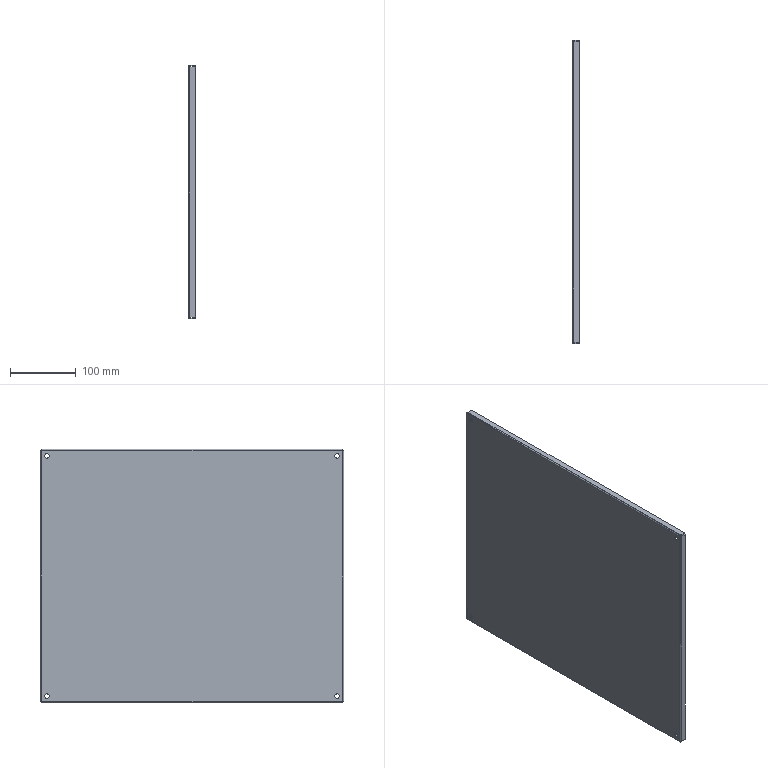Part | SolidWorks | features BaseBody 1 | 1 solid | 38 faces | box 10 x 462 x 386 mm | volume 287636 mm3 | plane 22 | cylinder 16 | commonest cylinder face diameters 7 x8 0.4 x4 3.4 x4
STEP:
#1=CARTESIAN_POINT('',(1256.5,54.,45.5));
#2=VERTEX_POINT('',#1);
#3=CARTESIAN_POINT('',(1256.5,54.,38.5));
#4=VERTEX_POINT('',#3);
#5=CARTESIAN_POINT('',(1256.5,54.,42.));
#6=DIRECTION('',(1.,0.,0.));
#7=DIRECTION('',(0.,0.,-1.));
#8=AXIS2_PLACEMENT_3D('',#5,#6,#7);
#9=CIRCLE('',#8,3.5);
#10=EDGE_CURVE('',#2,#4,#9,.T.);
#11=ORIENTED_EDGE('',*,*,#10,.T.);
#12=CARTESIAN_POINT('',(1255.,54.,38.5));
#13=VERTEX_POINT('',#12);
#14=CARTESIAN_POINT('',(1255.,54.,38.5));
#15=DIRECTION('',(-1.,0.,0.));
#16=VECTOR('',#15,1000.);
#17=LINE('',#14,#16);
#18=EDGE_CURVE('',#4,#13,#17,.T.);
#19=ORIENTED_EDGE('',*,*,#18,.T.);
#20=CARTESIAN_POINT('',(1255.,54.,45.5));
#21=VERTEX_POINT('',#20);
#22=CARTESIAN_POINT('',(1255.,54.,42.));
#23=DIRECTION('',(-1.,0.,0.));
#24=DIRECTION('',(0.,0.,-1.));
#25=AXIS2_PLACEMENT_3D('',#22,#23,#24);
#26=CIRCLE('',#25,3.5);
#27=EDGE_CURVE('',#13,#21,#26,.T.);
#28=ORIENTED_EDGE('',*,*,#27,.T.);
#29=CARTESIAN_POINT('',(1255.,54.,45.5));
#30=DIRECTION('',(-1.,0.,0.));
#31=VECTOR('',#30,1000.);
#32=LINE('',#29,#31);
#33=EDGE_CURVE('',#2,#21,#32,.T.);
#34=ORIENTED_EDGE('',*,*,#33,.F.);
#35=EDGE_LOOP('',(#11,#19,#28,#34));
#36=FACE_OUTER_BOUND('',#35,.T.);
#37=CARTESIAN_POINT('',(1255.,54.,42.));
#38=DIRECTION('',(-1.,0.,0.));
#39=DIRECTION('',(0.,0.,1.));
#40=AXIS2_PLACEMENT_3D('',#37,#38,#39);
#41=CYLINDRICAL_SURFACE('',#40,3.5);
#42=ADVANCED_FACE('',(#36),#41,.F.);
#43=CARTESIAN_POINT('',(1256.5,496.,411.5));
#44=VERTEX_POINT('',#43);
#45=CARTESIAN_POINT('',(1256.5,496.,404.5));
#46=VERTEX_POINT('',#45);
#47=CARTESIAN_POINT('',(1256.5,496.,408.));
#48=DIRECTION('',(1.,0.,0.));
#49=DIRECTION('',(0.,0.,-1.));
#50=AXIS2_PLACEMENT_3D('',#47,#48,#49);
#51=CIRCLE('',#50,3.5);
#52=EDGE_CURVE('',#44,#46,#51,.T.);
#53=ORIENTED_EDGE('',*,*,#52,.T.);
#54=CARTESIAN_POINT('',(1255.,496.,404.5));
#55=VERTEX_POINT('',#54);
#56=CARTESIAN_POINT('',(1255.,496.,404.5));
#57=DIRECTION('',(-1.,0.,0.));
#58=VECTOR('',#57,1000.);
#59=LINE('',#56,#58);
#60=EDGE_CURVE('',#46,#55,#59,.T.);
#61=ORIENTED_EDGE('',*,*,#60,.T.);
#62=CARTESIAN_POINT('',(1255.,496.,411.5));
#63=VERTEX_POINT('',#62);
#64=CARTESIAN_POINT('',(1255.,496.,408.));
#65=DIRECTION('',(-1.,0.,0.));
#66=DIRECTION('',(0.,0.,-1.));
#67=AXIS2_PLACEMENT_3D('',#64,#65,#66);
#68=CIRCLE('',#67,3.5);
#69=EDGE_CURVE('',#55,#63,#68,.T.);
#70=ORIENTED_EDGE('',*,*,#69,.T.);
#71=CARTESIAN_POINT('',(1255.,496.,411.5));
#72=DIRECTION('',(-1.,0.,0.));
#73=VECTOR('',#72,1000.);
#74=LINE('',#71,#73);
#75=EDGE_CURVE('',#44,#63,#74,.T.);
#76=ORIENTED_EDGE('',*,*,#75,.F.);
#77=EDGE_LOOP('',(#53,#61,#70,#76));
#78=FACE_OUTER_BOUND('',#77,.T.);
#79=CARTESIAN_POINT('',(1255.,496.,408.));
#80=DIRECTION('',(-1.,0.,0.));
#81=DIRECTION('',(0.,0.,1.));
#82=AXIS2_PLACEMENT_3D('',#79,#80,#81);
#83=CYLINDRICAL_SURFACE('',#82,3.5);
#84=ADVANCED_FACE('',(#78),#83,.F.);
#85=CARTESIAN_POINT('',(1256.5,54.,411.5));
#86=VERTEX_POINT('',#85);
#87=CARTESIAN_POINT('',(1256.5,54.,404.5));
#88=VERTEX_POINT('',#87);
#89=CARTESIAN_POINT('',(1256.5,54.,408.));
#90=DIRECTION('',(1.,0.,0.));
#91=DIRECTION('',(0.,0.,-1.));
#92=AXIS2_PLACEMENT_3D('',#89,#90,#91);
#93=CIRCLE('',#92,3.5);
#94=EDGE_CURVE('',#86,#88,#93,.T.);
#95=ORIENTED_EDGE('',*,*,#94,.T.);
#96=CARTESIAN_POINT('',(1255.,54.,404.5));
#97=VERTEX_POINT('',#96);
#98=CARTESIAN_POINT('',(1255.,54.,404.5));
#99=DIRECTION('',(-1.,0.,0.));
#100=VECTOR('',#99,1000.);
#101=LINE('',#98,#100);
#102=EDGE_CURVE('',#88,#97,#101,.T.);
#103=ORIENTED_EDGE('',*,*,#102,.T.);
#104=CARTESIAN_POINT('',(1255.,54.,411.5));
#105=VERTEX_POINT('',#104);
#106=CARTESIAN_POINT('',(1255.,54.,408.));
#107=DIRECTION('',(-1.,0.,0.));
#108=DIRECTION('',(0.,0.,-1.));
#109=AXIS2_PLACEMENT_3D('',#106,#107,#108);
#110=CIRCLE('',#109,3.5);
#111=EDGE_CURVE('',#97,#105,#110,.T.);
#112=ORIENTED_EDGE('',*,*,#111,.T.);
#113=CARTESIAN_POINT('',(1255.,54.,411.5));
#114=DIRECTION('',(-1.,0.,0.));
#115=VECTOR('',#114,1000.);
#116=LINE('',#113,#115);
#117=EDGE_CURVE('',#86,#105,#116,.T.);
#118=ORIENTED_EDGE('',*,*,#117,.F.);
#119=EDGE_LOOP('',(#95,#103,#112,#118));
#120=FACE_OUTER_BOUND('',#119,.T.);
#121=CARTESIAN_POINT('',(1255.,54.,408.));
#122=DIRECTION('',(-1.,0.,0.));
#123=DIRECTION('',(0.,0.,1.));
#124=AXIS2_PLACEMENT_3D('',#121,#122,#123);
#125=CYLINDRICAL_SURFACE('',#124,3.5);
#126=ADVANCED_FACE('',(#120),#125,.F.);
#127=CARTESIAN_POINT('',(1256.5,496.,45.5));
#128=VERTEX_POINT('',#127);
#129=CARTESIAN_POINT('',(1256.5,496.,38.5));
#130=VERTEX_POINT('',#129);
#131=CARTESIAN_POINT('',(1256.5,496.,42.));
#132=DIRECTION('',(1.,0.,0.));
#133=DIRECTION('',(0.,0.,-1.));
#134=AXIS2_PLACEMENT_3D('',#131,#132,#133);
#135=CIRCLE('',#134,3.5);
#136=EDGE_CURVE('',#128,#130,#135,.T.);
#137=ORIENTED_EDGE('',*,*,#136,.T.);
#138=CARTESIAN_POINT('',(1255.,496.,38.5));
#139=VERTEX_POINT('',#138);
#140=CARTESIAN_POINT('',(1255.,496.,38.5));
#141=DIRECTION('',(-1.,0.,0.));
#142=VECTOR('',#141,1000.);
#143=LINE('',#140,#142);
#144=EDGE_CURVE('',#130,#139,#143,.T.);
#145=ORIENTED_EDGE('',*,*,#144,.T.);
#146=CARTESIAN_POINT('',(1255.,496.,45.5));
#147=VERTEX_POINT('',#146);
#148=CARTESIAN_POINT('',(1255.,496.,42.));
#149=DIRECTION('',(-1.,0.,0.));
#150=DIRECTION('',(0.,0.,-1.));
#151=AXIS2_PLACEMENT_3D('',#148,#149,#150);
#152=CIRCLE('',#151,3.5);
#153=EDGE_CURVE('',#139,#147,#152,.T.);
#154=ORIENTED_EDGE('',*,*,#153,.T.);
#155=CARTESIAN_POINT('',(1255.,496.,45.5));
#156=DIRECTION('',(-1.,0.,0.));
#157=VECTOR('',#156,1000.);
#158=LINE('',#155,#157);
#159=EDGE_CURVE('',#128,#147,#158,.T.);
#160=ORIENTED_EDGE('',*,*,#159,.F.);
#161=EDGE_LOOP('',(#137,#145,#154,#160));
#162=FACE_OUTER_BOUND('',#161,.T.);
#163=CARTESIAN_POINT('',(1255.,496.,42.));
#164=DIRECTION('',(-1.,0.,0.));
#165=DIRECTION('',(0.,0.,1.));
#166=AXIS2_PLACEMENT_3D('',#163,#164,#165);
#167=CYLINDRICAL_SURFACE('',#166,3.5);
#168=ADVANCED_FACE('',(#162),#167,.F.);
#169=CARTESIAN_POINT('',(1256.7,45.5,416.));
#170=VERTEX_POINT('',#169);
#171=CARTESIAN_POINT('',(1256.5,45.7,416.));
#172=VERTEX_POINT('',#171);
#173=CARTESIAN_POINT('',(1256.7,45.7,416.));
#174=DIRECTION('',(0.,0.,-1.));
#175=DIRECTION('',(0.,1.,0.));
#176=AXIS2_PLACEMENT_3D('',#173,#174,#175);
#177=CIRCLE('',#176,0.2);
#178=EDGE_CURVE('',#170,#172,#177,.T.);
#179=ORIENTED_EDGE('',*,*,#178,.F.);
#180=CARTESIAN_POINT('',(1256.7,45.5,34.));
#181=VERTEX_POINT('',#180);
#182=CARTESIAN_POINT('',(1256.7,45.5,416.));
#183=DIRECTION('',(0.,0.,1.));
#184=VECTOR('',#183,1000.);
#185=LINE('',#182,#184);
#186=EDGE_CURVE('',#181,#170,#185,.T.);
#187=ORIENTED_EDGE('',*,*,#186,.F.);
#188=CARTESIAN_POINT('',(1256.5,45.7,34.));
#189=VERTEX_POINT('',#188);
#190=CARTESIAN_POINT('',(1256.7,45.7,34.));
#191=DIRECTION('',(0.,0.,1.));
#192=DIRECTION('',(0.,1.,0.));
#193=AXIS2_PLACEMENT_3D('',#190,#191,#192);
#194=CIRCLE('',#193,0.2);
#195=EDGE_CURVE('',#189,#181,#194,.T.);
#196=ORIENTED_EDGE('',*,*,#195,.F.);
#197=CARTESIAN_POINT('',(1256.5,45.7,416.));
#198=DIRECTION('',(0.,0.,-1.));
#199=VECTOR('',#198,1000.);
#200=LINE('',#197,#199);
#201=EDGE_CURVE('',#172,#189,#200,.T.);
#202=ORIENTED_EDGE('',*,*,#201,.F.);
#203=EDGE_LOOP('',(#179,#187,#196,#202));
#204=FACE_OUTER_BOUND('',#203,.T.);
#205=CARTESIAN_POINT('',(1256.7,45.7,1023.809));
#206=DIRECTION('',(0.,0.,-1.));
#207=DIRECTION('',(0.,1.,0.));
#208=AXIS2_PLACEMENT_3D('',#205,#206,#207);
#209=CYLINDRICAL_SURFACE('',#208,0.2);
#210=ADVANCED_FACE('',(#204),#209,.F.);
#211=CARTESIAN_POINT('',(1256.7,44.,416.));
#212=VERTEX_POINT('',#211);
#213=CARTESIAN_POINT('',(1255.,45.7,416.));
#214=VERTEX_POINT('',#213);
#215=CARTESIAN_POINT('',(1256.7,45.7,416.));
#216=DIRECTION('',(0.,0.,-1.));
#217=DIRECTION('',(0.,1.,0.));
#218=AXIS2_PLACEMENT_3D('',#215,#216,#217);
#219=CIRCLE('',#218,1.7);
#220=EDGE_CURVE('',#212,#214,#219,.T.);
#221=ORIENTED_EDGE('',*,*,#220,.T.);
#222=CARTESIAN_POINT('',(1255.,45.7,34.));
#223=VERTEX_POINT('',#222);
#224=CARTESIAN_POINT('',(1255.,45.7,416.));
#225=DIRECTION('',(0.,0.,-1.));
#226=VECTOR('',#225,1000.);
#227=LINE('',#224,#226);
#228=EDGE_CURVE('',#214,#223,#227,.T.);
#229=ORIENTED_EDGE('',*,*,#228,.T.);
#230=CARTESIAN_POINT('',(1256.7,44.,34.));
#231=VERTEX_POINT('',#230);
#232=CARTESIAN_POINT('',(1256.7,45.7,34.));
#233=DIRECTION('',(0.,0.,1.));
#234=DIRECTION('',(0.,1.,0.));
#235=AXIS2_PLACEMENT_3D('',#232,#233,#234);
#236=CIRCLE('',#235,1.7);
#237=EDGE_CURVE('',#223,#231,#236,.T.);
#238=ORIENTED_EDGE('',*,*,#237,.T.);
#239=CARTESIAN_POINT('',(1256.7,44.,416.));
#240=DIRECTION('',(0.,0.,1.));
#241=VECTOR('',#240,1000.);
#242=LINE('',#239,#241);
#243=EDGE_CURVE('',#231,#212,#242,.T.);
#244=ORIENTED_EDGE('',*,*,#243,.T.);
#245=EDGE_LOOP('',(#221,#229,#238,#244));
#246=FACE_OUTER_BOUND('',#245,.T.);
#247=CARTESIAN_POINT('',(1256.7,45.7,1023.809));
#248=DIRECTION('',(0.,0.,-1.));
#249=DIRECTION('',(0.,1.,0.));
#250=AXIS2_PLACEMENT_3D('',#247,#248,#249);
#251=CYLINDRICAL_SURFACE('',#250,1.7);
#252=ADVANCED_FACE('',(#246),#251,.T.);
#253=CARTESIAN_POINT('',(1256.7,46.,33.5));
#254=VERTEX_POINT('',#253);
#255=CARTESIAN_POINT('',(1256.5,46.,33.7));
#256=VERTEX_POINT('',#255);
#257=CARTESIAN_POINT('',(1256.7,46.,33.7));
#258=DIRECTION('',(0.,1.,0.));
#259=DIRECTION('',(0.,0.,1.));
#260=AXIS2_PLACEMENT_3D('',#257,#258,#259);
#261=CIRCLE('',#260,0.2);
#262=EDGE_CURVE('',#254,#256,#261,.T.);
#263=ORIENTED_EDGE('',*,*,#262,.F.);
#264=CARTESIAN_POINT('',(1256.7,504.,33.5));
#265=VERTEX_POINT('',#264);
#266=CARTESIAN_POINT('',(1256.7,46.,33.5));
#267=DIRECTION('',(0.,-1.,0.));
#268=VECTOR('',#267,1000.);
#269=LINE('',#266,#268);
#270=EDGE_CURVE('',#265,#254,#269,.T.);
#271=ORIENTED_EDGE('',*,*,#270,.F.);
#272=CARTESIAN_POINT('',(1256.5,504.,33.7));
#273=VERTEX_POINT('',#272);
#274=CARTESIAN_POINT('',(1256.7,504.,33.7));
#275=DIRECTION('',(0.,-1.,0.));
#276=DIRECTION('',(0.,0.,1.));
#277=AXIS2_PLACEMENT_3D('',#274,#275,#276);
#278=CIRCLE('',#277,0.2);
#279=EDGE_CURVE('',#273,#265,#278,.T.);
#280=ORIENTED_EDGE('',*,*,#279,.F.);
#281=CARTESIAN_POINT('',(1256.5,46.,33.7));
#282=DIRECTION('',(0.,1.,0.));
#283=VECTOR('',#282,1000.);
#284=LINE('',#281,#283);
#285=EDGE_CURVE('',#256,#273,#284,.T.);
#286=ORIENTED_EDGE('',*,*,#285,.F.);
#287=EDGE_LOOP('',(#263,#271,#280,#286));
#288=FACE_OUTER_BOUND('',#287,.T.);
#289=CARTESIAN_POINT('',(1256.7,-566.536,33.7));
#290=DIRECTION('',(0.,1.,0.));
#291=DIRECTION('',(0.,0.,1.));
#292=AXIS2_PLACEMENT_3D('',#289,#290,#291);
#293=CYLINDRICAL_SURFACE('',#292,0.2);
#294=ADVANCED_FACE('',(#288),#293,.F.);
#295=CARTESIAN_POINT('',(1256.7,46.,32.));
#296=VERTEX_POINT('',#295);
#297=CARTESIAN_POINT('',(1255.,46.,33.7));
#298=VERTEX_POINT('',#297);
#299=CARTESIAN_POINT('',(1256.7,46.,33.7));
#300=DIRECTION('',(0.,1.,0.));
#301=DIRECTION('',(0.,0.,1.));
#302=AXIS2_PLACEMENT_3D('',#299,#300,#301);
#303=CIRCLE('',#302,1.7);
#304=EDGE_CURVE('',#296,#298,#303,.T.);
#305=ORIENTED_EDGE('',*,*,#304,.T.);
#306=CARTESIAN_POINT('',(1255.,504.,33.7));
#307=VERTEX_POINT('',#306);
#308=CARTESIAN_POINT('',(1255.,46.,33.7));
#309=DIRECTION('',(0.,1.,0.));
#310=VECTOR('',#309,1000.);
#311=LINE('',#308,#310);
#312=EDGE_CURVE('',#298,#307,#311,.T.);
#313=ORIENTED_EDGE('',*,*,#312,.T.);
#314=CARTESIAN_POINT('',(1256.7,504.,32.));
#315=VERTEX_POINT('',#314);
#316=CARTESIAN_POINT('',(1256.7,504.,33.7));
#317=DIRECTION('',(0.,-1.,0.));
#318=DIRECTION('',(0.,0.,1.));
#319=AXIS2_PLACEMENT_3D('',#316,#317,#318);
#320=CIRCLE('',#319,1.7);
#321=EDGE_CURVE('',#307,#315,#320,.T.);
#322=ORIENTED_EDGE('',*,*,#321,.T.);
#323=CARTESIAN_POINT('',(1256.7,46.,32.));
#324=DIRECTION('',(0.,-1.,0.));
#325=VECTOR('',#324,1000.);
#326=LINE('',#323,#325);
#327=EDGE_CURVE('',#315,#296,#326,.T.);
#328=ORIENTED_EDGE('',*,*,#327,.T.);
#329=EDGE_LOOP('',(#305,#313,#322,#328));
#330=FACE_OUTER_BOUND('',#329,.T.);
#331=CARTESIAN_POINT('',(1256.7,-566.536,33.7));
#332=DIRECTION('',(0.,1.,0.));
#333=DIRECTION('',(0.,0.,1.));
#334=AXIS2_PLACEMENT_3D('',#331,#332,#333);
#335=CYLINDRICAL_SURFACE('',#334,1.7);
#336=ADVANCED_FACE('',(#330),#335,.T.);
#337=CARTESIAN_POINT('',(1256.7,504.5,34.));
#338=VERTEX_POINT('',#337);
#339=CARTESIAN_POINT('',(1256.5,504.3,34.));
#340=VERTEX_POINT('',#339);
#341=CARTESIAN_POINT('',(1256.7,504.3,34.));
#342=DIRECTION('',(0.,0.,1.));
#343=DIRECTION('',(1.,0.,0.));
#344=AXIS2_PLACEMENT_3D('',#341,#342,#343);
#345=CIRCLE('',#344,0.2);
#346=EDGE_CURVE('',#338,#340,#345,.T.);
#347=ORIENTED_EDGE('',*,*,#346,.F.);
#348=CARTESIAN_POINT('',(1256.7,504.5,416.));
#349=VERTEX_POINT('',#348);
#350=CARTESIAN_POINT('',(1256.7,504.5,34.));
#351=DIRECTION('',(0.,0.,-1.));
#352=VECTOR('',#351,1000.);
#353=LINE('',#350,#352);
#354=EDGE_CURVE('',#349,#338,#353,.T.);
#355=ORIENTED_EDGE('',*,*,#354,.F.);
#356=CARTESIAN_POINT('',(1256.5,504.3,416.));
#357=VERTEX_POINT('',#356);
#358=CARTESIAN_POINT('',(1256.7,504.3,416.));
#359=DIRECTION('',(0.,0.,-1.));
#360=DIRECTION('',(1.,0.,0.));
#361=AXIS2_PLACEMENT_3D('',#358,#359,#360);
#362=CIRCLE('',#361,0.2);
#363=EDGE_CURVE('',#357,#349,#362,.T.);
#364=ORIENTED_EDGE('',*,*,#363,.F.);
#365=CARTESIAN_POINT('',(1256.5,504.3,34.));
#366=DIRECTION('',(0.,0.,1.));
#367=VECTOR('',#366,1000.);
#368=LINE('',#365,#367);
#369=EDGE_CURVE('',#340,#357,#368,.T.);
#370=ORIENTED_EDGE('',*,*,#369,.F.);
#371=EDGE_LOOP('',(#347,#355,#364,#370));
#372=FACE_OUTER_BOUND('',#371,.T.);
#373=CARTESIAN_POINT('',(1256.7,504.3,-584.225));
#374=DIRECTION('',(0.,0.,1.));
#375=DIRECTION('',(1.,0.,0.));
#376=AXIS2_PLACEMENT_3D('',#373,#374,#375);
#377=CYLINDRICAL_SURFACE('',#376,0.2);
#378=ADVANCED_FACE('',(#372),#377,.F.);
#379=CARTESIAN_POINT('',(1256.7,506.,34.));
#380=VERTEX_POINT('',#379);
#381=CARTESIAN_POINT('',(1255.,504.3,34.));
#382=VERTEX_POINT('',#381);
#383=CARTESIAN_POINT('',(1256.7,504.3,34.));
#384=DIRECTION('',(0.,0.,1.));
#385=DIRECTION('',(1.,0.,0.));
#386=AXIS2_PLACEMENT_3D('',#383,#384,#385);
#387=CIRCLE('',#386,1.7);
#388=EDGE_CURVE('',#380,#382,#387,.T.);
#389=ORIENTED_EDGE('',*,*,#388,.T.);
#390=CARTESIAN_POINT('',(1255.,504.3,416.));
#391=VERTEX_POINT('',#390);
#392=CARTESIAN_POINT('',(1255.,504.3,34.));
#393=DIRECTION('',(0.,0.,1.));
#394=VECTOR('',#393,1000.);
#395=LINE('',#392,#394);
#396=EDGE_CURVE('',#382,#391,#395,.T.);
#397=ORIENTED_EDGE('',*,*,#396,.T.);
#398=CARTESIAN_POINT('',(1256.7,506.,416.));
#399=VERTEX_POINT('',#398);
#400=CARTESIAN_POINT('',(1256.7,504.3,416.));
#401=DIRECTION('',(0.,0.,-1.));
#402=DIRECTION('',(1.,0.,0.));
#403=AXIS2_PLACEMENT_3D('',#400,#401,#402);
#404=CIRCLE('',#403,1.7);
#405=EDGE_CURVE('',#391,#399,#404,.T.);
#406=ORIENTED_EDGE('',*,*,#405,.T.);
#407=CARTESIAN_POINT('',(1256.7,506.,34.));
#408=DIRECTION('',(0.,0.,-1.));
#409=VECTOR('',#408,1000.);
#410=LINE('',#407,#409);
#411=EDGE_CURVE('',#399,#380,#410,.T.);
#412=ORIENTED_EDGE('',*,*,#411,.T.);
#413=EDGE_LOOP('',(#389,#397,#406,#412));
#414=FACE_OUTER_BOUND('',#413,.T.);
#415=CARTESIAN_POINT('',(1256.7,504.3,-584.225));
#416=DIRECTION('',(0.,0.,1.));
#417=DIRECTION('',(1.,0.,0.));
#418=AXIS2_PLACEMENT_3D('',#415,#416,#417);
#419=CYLINDRICAL_SURFACE('',#418,1.7);
#420=ADVANCED_FACE('',(#414),#419,.T.);
#421=CARTESIAN_POINT('',(1256.7,504.,416.5));
#422=VERTEX_POINT('',#421);
#423=CARTESIAN_POINT('',(1256.5,504.,416.3));
#424=VERTEX_POINT('',#423);
#425=CARTESIAN_POINT('',(1256.7,504.,416.3));
#426=DIRECTION('',(0.,-1.,0.));
#427=DIRECTION('',(0.,0.,-1.));
#428=AXIS2_PLACEMENT_3D('',#425,#426,#427);
#429=CIRCLE('',#428,0.2);
#430=EDGE_CURVE('',#422,#424,#429,.T.);
#431=ORIENTED_EDGE('',*,*,#430,.F.);
#432=CARTESIAN_POINT('',(1256.7,46.,416.5));
#433=VERTEX_POINT('',#432);
#434=CARTESIAN_POINT('',(1256.7,504.,416.5));
#435=DIRECTION('',(0.,1.,0.));
#436=VECTOR('',#435,1000.);
#437=LINE('',#434,#436);
#438=EDGE_CURVE('',#433,#422,#437,.T.);
#439=ORIENTED_EDGE('',*,*,#438,.F.);
#440=CARTESIAN_POINT('',(1256.5,46.,416.3));
#441=VERTEX_POINT('',#440);
#442=CARTESIAN_POINT('',(1256.7,46.,416.3));
#443=DIRECTION('',(0.,1.,0.));
#444=DIRECTION('',(0.,0.,-1.));
#445=AXIS2_PLACEMENT_3D('',#442,#443,#444);
#446=CIRCLE('',#445,0.2);
#447=EDGE_CURVE('',#441,#433,#446,.T.);
#448=ORIENTED_EDGE('',*,*,#447,.F.);
#449=CARTESIAN_POINT('',(1256.5,504.,416.3));
#450=DIRECTION('',(0.,-1.,0.));
#451=VECTOR('',#450,1000.);
#452=LINE('',#449,#451);
#453=EDGE_CURVE('',#424,#441,#452,.T.);
#454=ORIENTED_EDGE('',*,*,#453,.F.);
#455=EDGE_LOOP('',(#431,#439,#448,#454));
#456=FACE_OUTER_BOUND('',#455,.T.);
#457=CARTESIAN_POINT('',(1256.7,1126.881,416.3));
#458=DIRECTION('',(0.,-1.,0.));
#459=DIRECTION('',(0.,0.,-1.));
#460=AXIS2_PLACEMENT_3D('',#457,#458,#459);
#461=CYLINDRICAL_SURFACE('',#460,0.2);
#462=ADVANCED_FACE('',(#456),#461,.F.);
#463=CARTESIAN_POINT('',(1256.7,504.,418.));
#464=VERTEX_POINT('',#463);
#465=CARTESIAN_POINT('',(1255.,504.,416.3));
#466=VERTEX_POINT('',#465);
#467=CARTESIAN_POINT('',(1256.7,504.,416.3));
#468=DIRECTION('',(0.,-1.,0.));
#469=DIRECTION('',(0.,0.,-1.));
#470=AXIS2_PLACEMENT_3D('',#467,#468,#469);
#471=CIRCLE('',#470,1.7);
#472=EDGE_CURVE('',#464,#466,#471,.T.);
#473=ORIENTED_EDGE('',*,*,#472,.T.);
#474=CARTESIAN_POINT('',(1255.,46.,416.3));
#475=VERTEX_POINT('',#474);
#476=CARTESIAN_POINT('',(1255.,504.,416.3));
#477=DIRECTION('',(0.,-1.,0.));
#478=VECTOR('',#477,1000.);
#479=LINE('',#476,#478);
#480=EDGE_CURVE('',#466,#475,#479,.T.);
#481=ORIENTED_EDGE('',*,*,#480,.T.);
#482=CARTESIAN_POINT('',(1256.7,46.,418.));
#483=VERTEX_POINT('',#482);
#484=CARTESIAN_POINT('',(1256.7,46.,416.3));
#485=DIRECTION('',(0.,1.,0.));
#486=DIRECTION('',(0.,0.,-1.));
#487=AXIS2_PLACEMENT_3D('',#484,#485,#486);
#488=CIRCLE('',#487,1.7);
#489=EDGE_CURVE('',#475,#483,#488,.T.);
#490=ORIENTED_EDGE('',*,*,#489,.T.);
#491=CARTESIAN_POINT('',(1256.7,504.,418.));
#492=DIRECTION('',(0.,1.,0.));
#493=VECTOR('',#492,1000.);
#494=LINE('',#491,#493);
#495=EDGE_CURVE('',#483,#464,#494,.T.);
#496=ORIENTED_EDGE('',*,*,#495,.T.);
#497=EDGE_LOOP('',(#473,#481,#490,#496));
#498=FACE_OUTER_BOUND('',#497,.T.);
#499=CARTESIAN_POINT('',(1256.7,1126.881,416.3));
#500=DIRECTION('',(0.,-1.,0.));
#501=DIRECTION('',(0.,0.,-1.));
#502=AXIS2_PLACEMENT_3D('',#499,#500,#501);
#503=CYLINDRICAL_SURFACE('',#502,1.7);
#504=ADVANCED_FACE('',(#498),#503,.T.);
#505=ORIENTED_EDGE('',*,*,#136,.F.);
#506=CARTESIAN_POINT('',(1256.5,496.,42.));
#507=DIRECTION('',(1.,0.,0.));
#508=DIRECTION('',(0.,0.,-1.));
#509=AXIS2_PLACEMENT_3D('',#506,#507,#508);
#510=CIRCLE('',#509,3.5);
#511=EDGE_CURVE('',#130,#128,#510,.T.);
#512=ORIENTED_EDGE('',*,*,#511,.F.);
#513=EDGE_LOOP('',(#505,#512));
#514=FACE_BOUND('',#513,.T.);
#515=ORIENTED_EDGE('',*,*,#94,.F.);
#516=CARTESIAN_POINT('',(1256.5,54.,408.));
#517=DIRECTION('',(1.,0.,0.));
#518=DIRECTION('',(0.,0.,-1.));
#519=AXIS2_PLACEMENT_3D('',#516,#517,#518);
#520=CIRCLE('',#519,3.5);
#521=EDGE_CURVE('',#88,#86,#520,.T.);
#522=ORIENTED_EDGE('',*,*,#521,.F.);
#523=EDGE_LOOP('',(#515,#522));
#524=FACE_BOUND('',#523,.T.);
#525=ORIENTED_EDGE('',*,*,#52,.F.);
#526=CARTESIAN_POINT('',(1256.5,496.,408.));
#527=DIRECTION('',(1.,0.,0.));
#528=DIRECTION('',(0.,0.,-1.));
#529=AXIS2_PLACEMENT_3D('',#526,#527,#528);
#530=CIRCLE('',#529,3.5);
#531=EDGE_CURVE('',#46,#44,#530,.T.);
#532=ORIENTED_EDGE('',*,*,#531,.F.);
#533=EDGE_LOOP('',(#525,#532));
#534=FACE_BOUND('',#533,.T.);
#535=ORIENTED_EDGE('',*,*,#10,.F.);
#536=CARTESIAN_POINT('',(1256.5,54.,42.));
#537=DIRECTION('',(1.,0.,0.));
#538=DIRECTION('',(0.,0.,-1.));
#539=AXIS2_PLACEMENT_3D('',#536,#537,#538);
#540=CIRCLE('',#539,3.5);
#541=EDGE_CURVE('',#4,#2,#540,.T.);
#542=ORIENTED_EDGE('',*,*,#541,.F.);
#543=EDGE_LOOP('',(#535,#542));
#544=FACE_BOUND('',#543,.T.);
#545=CARTESIAN_POINT('',(1256.5,46.,416.));
#546=VERTEX_POINT('',#545);
#547=CARTESIAN_POINT('',(1256.5,0.,416.));
#548=DIRECTION('',(0.,-1.,0.));
#549=VECTOR('',#548,1000.);
#550=LINE('',#547,#549);
#551=EDGE_CURVE('',#546,#172,#550,.T.);
#552=ORIENTED_EDGE('',*,*,#551,.T.);
#553=ORIENTED_EDGE('',*,*,#201,.T.);
#554=CARTESIAN_POINT('',(1256.5,46.,34.));
#555=VERTEX_POINT('',#554);
#556=CARTESIAN_POINT('',(1256.5,0.,34.));
#557=DIRECTION('',(0.,1.,0.));
#558=VECTOR('',#557,1000.);
#559=LINE('',#556,#558);
#560=EDGE_CURVE('',#189,#555,#559,.T.);
#561=ORIENTED_EDGE('',*,*,#560,.T.);
#562=CARTESIAN_POINT('',(1256.5,46.,0.));
#563=DIRECTION('',(0.,0.,-1.));
#564=VECTOR('',#563,1000.);
#565=LINE('',#562,#564);
#566=EDGE_CURVE('',#555,#256,#565,.T.);
#567=ORIENTED_EDGE('',*,*,#566,.T.);
#568=ORIENTED_EDGE('',*,*,#285,.T.);
#569=CARTESIAN_POINT('',(1256.5,504.,34.));
#570=VERTEX_POINT('',#569);
#571=CARTESIAN_POINT('',(1256.5,504.,0.));
#572=DIRECTION('',(0.,0.,1.));
#573=VECTOR('',#572,1000.);
#574=LINE('',#571,#573);
#575=EDGE_CURVE('',#273,#570,#574,.T.);
#576=ORIENTED_EDGE('',*,*,#575,.T.);
#577=CARTESIAN_POINT('',(1256.5,0.,34.));
#578=DIRECTION('',(0.,1.,0.));
#579=VECTOR('',#578,1000.);
#580=LINE('',#577,#579);
#581=EDGE_CURVE('',#570,#340,#580,.T.);
#582=ORIENTED_EDGE('',*,*,#581,.T.);
#583=ORIENTED_EDGE('',*,*,#369,.T.);
#584=CARTESIAN_POINT('',(1256.5,504.,416.));
#585=VERTEX_POINT('',#584);
#586=CARTESIAN_POINT('',(1256.5,0.,416.));
#587=DIRECTION('',(0.,-1.,0.));
#588=VECTOR('',#587,1000.);
#589=LINE('',#586,#588);
#590=EDGE_CURVE('',#357,#585,#589,.T.);
#591=ORIENTED_EDGE('',*,*,#590,.T.);
#592=CARTESIAN_POINT('',(1256.5,504.,0.));
#593=DIRECTION('',(0.,0.,1.));
#594=VECTOR('',#593,1000.);
#595=LINE('',#592,#594);
#596=EDGE_CURVE('',#585,#424,#595,.T.);
#597=ORIENTED_EDGE('',*,*,#596,.T.);
#598=ORIENTED_EDGE('',*,*,#453,.T.);
#599=CARTESIAN_POINT('',(1256.5,46.,0.));
#600=DIRECTION('',(0.,0.,-1.));
#601=VECTOR('',#600,1000.);
#602=LINE('',#599,#601);
#603=EDGE_CURVE('',#441,#546,#602,.T.);
#604=ORIENTED_EDGE('',*,*,#603,.T.);
#605=EDGE_LOOP('',(#552,#553,#561,#567,#568,#576,#582,#583,#591,#597,#598,#604));
#606=FACE_OUTER_BOUND('',#605,.T.);
#607=CARTESIAN_POINT('',(1256.5,0.,0.));
#608=DIRECTION('',(1.,0.,0.));
#609=DIRECTION('',(0.,1.,0.));
#610=AXIS2_PLACEMENT_3D('',#607,#608,#609);
#611=PLANE('',#610);
#612=ADVANCED_FACE('',(#514,#524,#534,#544,#606),#611,.T.);
#613=CARTESIAN_POINT('',(1255.,496.,42.));
#614=DIRECTION('',(-1.,0.,0.));
#615=DIRECTION('',(0.,0.,-1.));
#616=AXIS2_PLACEMENT_3D('',#613,#614,#615);
#617=CIRCLE('',#616,3.5);
#618=EDGE_CURVE('',#147,#139,#617,.T.);
#619=ORIENTED_EDGE('',*,*,#618,.F.);
#620=ORIENTED_EDGE('',*,*,#153,.F.);
#621=EDGE_LOOP('',(#619,#620));
#622=FACE_BOUND('',#621,.T.);
#623=CARTESIAN_POINT('',(1255.,54.,408.));
#624=DIRECTION('',(-1.,0.,0.));
#625=DIRECTION('',(0.,0.,-1.));
#626=AXIS2_PLACEMENT_3D('',#623,#624,#625);
#627=CIRCLE('',#626,3.5);
#628=EDGE_CURVE('',#105,#97,#627,.T.);
#629=ORIENTED_EDGE('',*,*,#628,.F.);
#630=ORIENTED_EDGE('',*,*,#111,.F.);
#631=EDGE_LOOP('',(#629,#630));
#632=FACE_BOUND('',#631,.T.);
#633=CARTESIAN_POINT('',(1255.,496.,408.));
#634=DIRECTION('',(-1.,0.,0.));
#635=DIRECTION('',(0.,0.,-1.));
#636=AXIS2_PLACEMENT_3D('',#633,#634,#635);
#637=CIRCLE('',#636,3.5);
#638=EDGE_CURVE('',#63,#55,#637,.T.);
#639=ORIENTED_EDGE('',*,*,#638,.F.);
#640=ORIENTED_EDGE('',*,*,#69,.F.);
#641=EDGE_LOOP('',(#639,#640));
#642=FACE_BOUND('',#641,.T.);
#643=CARTESIAN_POINT('',(1255.,54.,42.));
#644=DIRECTION('',(-1.,0.,0.));
#645=DIRECTION('',(0.,0.,-1.));
#646=AXIS2_PLACEMENT_3D('',#643,#644,#645);
#647=CIRCLE('',#646,3.5);
#648=EDGE_CURVE('',#21,#13,#647,.T.);
#649=ORIENTED_EDGE('',*,*,#648,.F.);
#650=ORIENTED_EDGE('',*,*,#27,.F.);
#651=EDGE_LOOP('',(#649,#650));
#652=FACE_BOUND('',#651,.T.);
#653=ORIENTED_EDGE('',*,*,#228,.F.);
#654=CARTESIAN_POINT('',(1255.,46.,416.));
#655=VERTEX_POINT('',#654);
#656=CARTESIAN_POINT('',(1255.,0.,416.));
#657=DIRECTION('',(0.,-1.,0.));
#658=VECTOR('',#657,1000.);
#659=LINE('',#656,#658);
#660=EDGE_CURVE('',#655,#214,#659,.T.);
#661=ORIENTED_EDGE('',*,*,#660,.F.);
#662=CARTESIAN_POINT('',(1255.,46.,0.));
#663=DIRECTION('',(0.,0.,-1.));
#664=VECTOR('',#663,1000.);
#665=LINE('',#662,#664);
#666=EDGE_CURVE('',#475,#655,#665,.T.);
#667=ORIENTED_EDGE('',*,*,#666,.F.);
#668=ORIENTED_EDGE('',*,*,#480,.F.);
#669=CARTESIAN_POINT('',(1255.,504.,416.));
#670=VERTEX_POINT('',#669);
#671=CARTESIAN_POINT('',(1255.,504.,0.));
#672=DIRECTION('',(0.,0.,1.));
#673=VECTOR('',#672,1000.);
#674=LINE('',#671,#673);
#675=EDGE_CURVE('',#670,#466,#674,.T.);
#676=ORIENTED_EDGE('',*,*,#675,.F.);
#677=CARTESIAN_POINT('',(1255.,0.,416.));
#678=DIRECTION('',(0.,-1.,0.));
#679=VECTOR('',#678,1000.);
#680=LINE('',#677,#679);
#681=EDGE_CURVE('',#391,#670,#680,.T.);
#682=ORIENTED_EDGE('',*,*,#681,.F.);
#683=ORIENTED_EDGE('',*,*,#396,.F.);
#684=CARTESIAN_POINT('',(1255.,504.,34.));
#685=VERTEX_POINT('',#684);
#686=CARTESIAN_POINT('',(1255.,0.,34.));
#687=DIRECTION('',(0.,1.,0.));
#688=VECTOR('',#687,1000.);
#689=LINE('',#686,#688);
#690=EDGE_CURVE('',#685,#382,#689,.T.);
#691=ORIENTED_EDGE('',*,*,#690,.F.);
#692=CARTESIAN_POINT('',(1255.,504.,0.));
#693=DIRECTION('',(0.,0.,1.));
#694=VECTOR('',#693,1000.);
#695=LINE('',#692,#694);
#696=EDGE_CURVE('',#307,#685,#695,.T.);
#697=ORIENTED_EDGE('',*,*,#696,.F.);
#698=ORIENTED_EDGE('',*,*,#312,.F.);
#699=CARTESIAN_POINT('',(1255.,46.,34.));
#700=VERTEX_POINT('',#699);
#701=CARTESIAN_POINT('',(1255.,46.,0.));
#702=DIRECTION('',(0.,0.,-1.));
#703=VECTOR('',#702,1000.);
#704=LINE('',#701,#703);
#705=EDGE_CURVE('',#700,#298,#704,.T.);
#706=ORIENTED_EDGE('',*,*,#705,.F.);
#707=CARTESIAN_POINT('',(1255.,0.,34.));
#708=DIRECTION('',(0.,1.,0.));
#709=VECTOR('',#708,1000.);
#710=LINE('',#707,#709);
#711=EDGE_CURVE('',#223,#700,#710,.T.);
#712=ORIENTED_EDGE('',*,*,#711,.F.);
#713=EDGE_LOOP('',(#653,#661,#667,#668,#676,#682,#683,#691,#697,#698,#706,#712));
#714=FACE_OUTER_BOUND('',#713,.T.);
#715=CARTESIAN_POINT('',(1255.,0.,0.));
#716=DIRECTION('',(1.,0.,0.));
#717=DIRECTION('',(0.,1.,0.));
#718=AXIS2_PLACEMENT_3D('',#715,#716,#717);
#719=PLANE('',#718);
#720=ADVANCED_FACE('',(#622,#632,#642,#652,#714),#719,.F.);
#721=CARTESIAN_POINT('',(1265.,46.,416.5));
#722=VERTEX_POINT('',#721);
#723=CARTESIAN_POINT('',(643.109,46.,416.5));
#724=DIRECTION('',(-1.,0.,0.));
#725=VECTOR('',#724,1000.);
#726=LINE('',#723,#725);
#727=EDGE_CURVE('',#722,#433,#726,.T.);
#728=ORIENTED_EDGE('',*,*,#727,.T.);
#729=ORIENTED_EDGE('',*,*,#438,.T.);
#730=CARTESIAN_POINT('',(1265.,504.,416.5));
#731=VERTEX_POINT('',#730);
#732=CARTESIAN_POINT('',(643.109,504.,416.5));
#733=DIRECTION('',(1.,0.,0.));
#734=VECTOR('',#733,1000.);
#735=LINE('',#732,#734);
#736=EDGE_CURVE('',#422,#731,#735,.T.);
#737=ORIENTED_EDGE('',*,*,#736,.T.);
#738=CARTESIAN_POINT('',(1265.,509.5,416.5));
#739=DIRECTION('',(0.,-1.,0.));
#740=VECTOR('',#739,1000.);
#741=LINE('',#738,#740);
#742=EDGE_CURVE('',#731,#722,#741,.T.);
#743=ORIENTED_EDGE('',*,*,#742,.T.);
#744=EDGE_LOOP('',(#728,#729,#737,#743));
#745=FACE_OUTER_BOUND('',#744,.T.);
#746=CARTESIAN_POINT('',(643.109,509.5,416.5));
#747=DIRECTION('',(0.,0.,1.));
#748=DIRECTION('',(1.,0.,0.));
#749=AXIS2_PLACEMENT_3D('',#746,#747,#748);
#750=PLANE('',#749);
#751=ADVANCED_FACE('',(#745),#750,.F.);
#752=CARTESIAN_POINT('',(1265.,46.,418.));
#753=VERTEX_POINT('',#752);
#754=CARTESIAN_POINT('',(643.109,46.,418.));
#755=DIRECTION('',(1.,0.,0.));
#756=VECTOR('',#755,1000.);
#757=LINE('',#754,#756);
#758=EDGE_CURVE('',#483,#753,#757,.T.);
#759=ORIENTED_EDGE('',*,*,#758,.F.);
#760=ORIENTED_EDGE('',*,*,#489,.F.);
#761=ORIENTED_EDGE('',*,*,#666,.T.);
#762=CARTESIAN_POINT('',(2449.482,46.,416.));
#763=DIRECTION('',(-1.,0.,0.));
#764=VECTOR('',#763,1000.);
#765=LINE('',#762,#764);
#766=EDGE_CURVE('',#546,#655,#765,.T.);
#767=ORIENTED_EDGE('',*,*,#766,.F.);
#768=ORIENTED_EDGE('',*,*,#603,.F.);
#769=ORIENTED_EDGE('',*,*,#447,.T.);
#770=ORIENTED_EDGE('',*,*,#727,.F.);
#771=CARTESIAN_POINT('',(1265.,46.,-498.15));
#772=DIRECTION('',(0.,0.,1.));
#773=VECTOR('',#772,1000.);
#774=LINE('',#771,#773);
#775=EDGE_CURVE('',#722,#753,#774,.T.);
#776=ORIENTED_EDGE('',*,*,#775,.T.);
#777=EDGE_LOOP('',(#759,#760,#761,#767,#768,#769,#770,#776));
#778=FACE_OUTER_BOUND('',#777,.T.);
#779=CARTESIAN_POINT('',(643.109,46.,-498.15));
#780=DIRECTION('',(0.,1.,0.));
#781=DIRECTION('',(1.,0.,0.));
#782=AXIS2_PLACEMENT_3D('',#779,#780,#781);
#783=PLANE('',#782);
#784=ADVANCED_FACE('',(#778),#783,.F.);
#785=ORIENTED_EDGE('',*,*,#495,.F.);
#786=ORIENTED_EDGE('',*,*,#758,.T.);
#787=CARTESIAN_POINT('',(1265.,504.,418.));
#788=VERTEX_POINT('',#787);
#789=CARTESIAN_POINT('',(1265.,511.,418.));
#790=DIRECTION('',(0.,1.,0.));
#791=VECTOR('',#790,1000.);
#792=LINE('',#789,#791);
#793=EDGE_CURVE('',#753,#788,#792,.T.);
#794=ORIENTED_EDGE('',*,*,#793,.T.);
#795=CARTESIAN_POINT('',(1253.672,504.,418.));
#796=DIRECTION('',(1.,0.,0.));
#797=VECTOR('',#796,1000.);
#798=LINE('',#795,#797);
#799=EDGE_CURVE('',#464,#788,#798,.T.);
#800=ORIENTED_EDGE('',*,*,#799,.F.);
#801=EDGE_LOOP('',(#785,#786,#794,#800));
#802=FACE_OUTER_BOUND('',#801,.T.);
#803=CARTESIAN_POINT('',(1265.,511.,418.));
#804=DIRECTION('',(0.,0.,1.));
#805=DIRECTION('',(1.,0.,0.));
#806=AXIS2_PLACEMENT_3D('',#803,#804,#805);
#807=PLANE('',#806);
#808=ADVANCED_FACE('',(#802),#807,.T.);
#809=ORIENTED_EDGE('',*,*,#799,.T.);
#810=CARTESIAN_POINT('',(1265.,504.,-498.15));
#811=DIRECTION('',(0.,0.,1.));
#812=VECTOR('',#811,1000.);
#813=LINE('',#810,#812);
#814=EDGE_CURVE('',#731,#788,#813,.T.);
#815=ORIENTED_EDGE('',*,*,#814,.F.);
#816=ORIENTED_EDGE('',*,*,#736,.F.);
#817=ORIENTED_EDGE('',*,*,#430,.T.);
#818=ORIENTED_EDGE('',*,*,#596,.F.);
#819=CARTESIAN_POINT('',(2449.482,504.,416.));
#820=DIRECTION('',(-1.,0.,0.));
#821=VECTOR('',#820,1000.);
#822=LINE('',#819,#821);
#823=EDGE_CURVE('',#585,#670,#822,.T.);
#824=ORIENTED_EDGE('',*,*,#823,.T.);
#825=ORIENTED_EDGE('',*,*,#675,.T.);
#826=ORIENTED_EDGE('',*,*,#472,.F.);
#827=EDGE_LOOP('',(#809,#815,#816,#817,#818,#824,#825,#826));
#828=FACE_OUTER_BOUND('',#827,.T.);
#829=CARTESIAN_POINT('',(643.109,504.,-498.15));
#830=DIRECTION('',(0.,-1.,0.));
#831=DIRECTION('',(0.,0.,-1.));
#832=AXIS2_PLACEMENT_3D('',#829,#830,#831);
#833=PLANE('',#832);
#834=ADVANCED_FACE('',(#828),#833,.F.);
#835=ORIENTED_EDGE('',*,*,#793,.F.);
#836=ORIENTED_EDGE('',*,*,#775,.F.);
#837=ORIENTED_EDGE('',*,*,#742,.F.);
#838=ORIENTED_EDGE('',*,*,#814,.T.);
#839=EDGE_LOOP('',(#835,#836,#837,#838));
#840=FACE_OUTER_BOUND('',#839,.T.);
#841=CARTESIAN_POINT('',(1265.,509.5,-498.15));
#842=DIRECTION('',(-1.,0.,0.));
#843=DIRECTION('',(0.,1.,0.));
#844=AXIS2_PLACEMENT_3D('',#841,#842,#843);
#845=PLANE('',#844);
#846=ADVANCED_FACE('',(#840),#845,.F.);
#847=CARTESIAN_POINT('',(1265.,504.5,416.));
#848=VERTEX_POINT('',#847);
#849=CARTESIAN_POINT('',(643.109,504.5,416.));
#850=DIRECTION('',(-1.,0.,0.));
#851=VECTOR('',#850,1000.);
#852=LINE('',#849,#851);
#853=EDGE_CURVE('',#848,#349,#852,.T.);
#854=ORIENTED_EDGE('',*,*,#853,.T.);
#855=ORIENTED_EDGE('',*,*,#354,.T.);
#856=CARTESIAN_POINT('',(1265.,504.5,34.));
#857=VERTEX_POINT('',#856);
#858=CARTESIAN_POINT('',(643.109,504.5,34.));
#859=DIRECTION('',(1.,0.,0.));
#860=VECTOR('',#859,1000.);
#861=LINE('',#858,#860);
#862=EDGE_CURVE('',#338,#857,#861,.T.);
#863=ORIENTED_EDGE('',*,*,#862,.T.);
#864=CARTESIAN_POINT('',(1265.,504.5,28.5));
#865=DIRECTION('',(0.,0.,1.));
#866=VECTOR('',#865,1000.);
#867=LINE('',#864,#866);
#868=EDGE_CURVE('',#857,#848,#867,.T.);
#869=ORIENTED_EDGE('',*,*,#868,.T.);
#870=EDGE_LOOP('',(#854,#855,#863,#869));
#871=FACE_OUTER_BOUND('',#870,.T.);
#872=CARTESIAN_POINT('',(643.109,504.5,28.5));
#873=DIRECTION('',(0.,1.,0.));
#874=DIRECTION('',(1.,0.,0.));
#875=AXIS2_PLACEMENT_3D('',#872,#873,#874);
#876=PLANE('',#875);
#877=ADVANCED_FACE('',(#871),#876,.F.);
#878=CARTESIAN_POINT('',(1265.,506.,416.));
#879=VERTEX_POINT('',#878);
#880=CARTESIAN_POINT('',(643.109,506.,416.));
#881=DIRECTION('',(1.,0.,0.));
#882=VECTOR('',#881,1000.);
#883=LINE('',#880,#882);
#884=EDGE_CURVE('',#399,#879,#883,.T.);
#885=ORIENTED_EDGE('',*,*,#884,.F.);
#886=ORIENTED_EDGE('',*,*,#405,.F.);
#887=ORIENTED_EDGE('',*,*,#681,.T.);
#888=ORIENTED_EDGE('',*,*,#823,.F.);
#889=ORIENTED_EDGE('',*,*,#590,.F.);
#890=ORIENTED_EDGE('',*,*,#363,.T.);
#891=ORIENTED_EDGE('',*,*,#853,.F.);
#892=CARTESIAN_POINT('',(1265.,-258.18,416.));
#893=DIRECTION('',(0.,1.,0.));
#894=VECTOR('',#893,1000.);
#895=LINE('',#892,#894);
#896=EDGE_CURVE('',#848,#879,#895,.T.);
#897=ORIENTED_EDGE('',*,*,#896,.T.);
#898=EDGE_LOOP('',(#885,#886,#887,#888,#889,#890,#891,#897));
#899=FACE_OUTER_BOUND('',#898,.T.);
#900=CARTESIAN_POINT('',(643.109,-258.18,416.));
#901=DIRECTION('',(0.,0.,-1.));
#902=DIRECTION('',(-1.,0.,0.));
#903=AXIS2_PLACEMENT_3D('',#900,#901,#902);
#904=PLANE('',#903);
#905=ADVANCED_FACE('',(#899),#904,.F.);
#906=ORIENTED_EDGE('',*,*,#411,.F.);
#907=ORIENTED_EDGE('',*,*,#884,.T.);
#908=CARTESIAN_POINT('',(1265.,506.,34.));
#909=VERTEX_POINT('',#908);
#910=CARTESIAN_POINT('',(1265.,506.,423.));
#911=DIRECTION('',(0.,0.,-1.));
#912=VECTOR('',#911,1000.);
#913=LINE('',#910,#912);
#914=EDGE_CURVE('',#879,#909,#913,.T.);
#915=ORIENTED_EDGE('',*,*,#914,.T.);
#916=CARTESIAN_POINT('',(1253.672,506.,34.));
#917=DIRECTION('',(1.,0.,0.));
#918=VECTOR('',#917,1000.);
#919=LINE('',#916,#918);
#920=EDGE_CURVE('',#380,#909,#919,.T.);
#921=ORIENTED_EDGE('',*,*,#920,.F.);
#922=EDGE_LOOP('',(#906,#907,#915,#921));
#923=FACE_OUTER_BOUND('',#922,.T.);
#924=CARTESIAN_POINT('',(1265.,506.,423.));
#925=DIRECTION('',(0.,1.,0.));
#926=DIRECTION('',(1.,0.,0.));
#927=AXIS2_PLACEMENT_3D('',#924,#925,#926);
#928=PLANE('',#927);
#929=ADVANCED_FACE('',(#923),#928,.T.);
#930=ORIENTED_EDGE('',*,*,#920,.T.);
#931=CARTESIAN_POINT('',(1265.,-258.18,34.));
#932=DIRECTION('',(0.,1.,0.));
#933=VECTOR('',#932,1000.);
#934=LINE('',#931,#933);
#935=EDGE_CURVE('',#857,#909,#934,.T.);
#936=ORIENTED_EDGE('',*,*,#935,.F.);
#937=ORIENTED_EDGE('',*,*,#862,.F.);
#938=ORIENTED_EDGE('',*,*,#346,.T.);
#939=ORIENTED_EDGE('',*,*,#581,.F.);
#940=CARTESIAN_POINT('',(2449.482,504.,34.));
#941=DIRECTION('',(-1.,0.,0.));
#942=VECTOR('',#941,1000.);
#943=LINE('',#940,#942);
#944=EDGE_CURVE('',#570,#685,#943,.T.);
#945=ORIENTED_EDGE('',*,*,#944,.T.);
#946=ORIENTED_EDGE('',*,*,#690,.T.);
#947=ORIENTED_EDGE('',*,*,#388,.F.);
#948=EDGE_LOOP('',(#930,#936,#937,#938,#939,#945,#946,#947));
#949=FACE_OUTER_BOUND('',#948,.T.);
#950=CARTESIAN_POINT('',(643.109,-258.18,34.));
#951=DIRECTION('',(0.,0.,1.));
#952=DIRECTION('',(1.,0.,0.));
#953=AXIS2_PLACEMENT_3D('',#950,#951,#952);
#954=PLANE('',#953);
#955=ADVANCED_FACE('',(#949),#954,.F.);
#956=ORIENTED_EDGE('',*,*,#914,.F.);
#957=ORIENTED_EDGE('',*,*,#896,.F.);
#958=ORIENTED_EDGE('',*,*,#868,.F.);
#959=ORIENTED_EDGE('',*,*,#935,.T.);
#960=EDGE_LOOP('',(#956,#957,#958,#959));
#961=FACE_OUTER_BOUND('',#960,.T.);
#962=CARTESIAN_POINT('',(1265.,-258.18,28.5));
#963=DIRECTION('',(-1.,0.,0.));
#964=DIRECTION('',(0.,0.,1.));
#965=AXIS2_PLACEMENT_3D('',#962,#963,#964);
#966=PLANE('',#965);
#967=ADVANCED_FACE('',(#961),#966,.F.);
#968=CARTESIAN_POINT('',(1265.,504.,33.5));
#969=VERTEX_POINT('',#968);
#970=CARTESIAN_POINT('',(643.109,504.,33.5));
#971=DIRECTION('',(-1.,0.,0.));
#972=VECTOR('',#971,1000.);
#973=LINE('',#970,#972);
#974=EDGE_CURVE('',#969,#265,#973,.T.);
#975=ORIENTED_EDGE('',*,*,#974,.T.);
#976=ORIENTED_EDGE('',*,*,#270,.T.);
#977=CARTESIAN_POINT('',(1265.,46.,33.5));
#978=VERTEX_POINT('',#977);
#979=CARTESIAN_POINT('',(643.109,46.,33.5));
#980=DIRECTION('',(1.,0.,0.));
#981=VECTOR('',#980,1000.);
#982=LINE('',#979,#981);
#983=EDGE_CURVE('',#254,#978,#982,.T.);
#984=ORIENTED_EDGE('',*,*,#983,.T.);
#985=CARTESIAN_POINT('',(1265.,40.5,33.5));
#986=DIRECTION('',(0.,1.,0.));
#987=VECTOR('',#986,1000.);
#988=LINE('',#985,#987);
#989=EDGE_CURVE('',#978,#969,#988,.T.);
#990=ORIENTED_EDGE('',*,*,#989,.T.);
#991=EDGE_LOOP('',(#975,#976,#984,#990));
#992=FACE_OUTER_BOUND('',#991,.T.);
#993=CARTESIAN_POINT('',(643.109,40.5,33.5));
#994=DIRECTION('',(0.,0.,-1.));
#995=DIRECTION('',(0.,-1.,0.));
#996=AXIS2_PLACEMENT_3D('',#993,#994,#995);
#997=PLANE('',#996);
#998=ADVANCED_FACE('',(#992),#997,.F.);
#999=CARTESIAN_POINT('',(1265.,504.,32.));
#1000=VERTEX_POINT('',#999);
#1001=CARTESIAN_POINT('',(643.109,504.,32.));
#1002=DIRECTION('',(1.,0.,0.));
#1003=VECTOR('',#1002,1000.);
#1004=LINE('',#1001,#1003);
#1005=EDGE_CURVE('',#315,#1000,#1004,.T.);
#1006=ORIENTED_EDGE('',*,*,#1005,.F.);
#1007=ORIENTED_EDGE('',*,*,#321,.F.);
#1008=ORIENTED_EDGE('',*,*,#696,.T.);
#1009=ORIENTED_EDGE('',*,*,#944,.F.);
#1010=ORIENTED_EDGE('',*,*,#575,.F.);
#1011=ORIENTED_EDGE('',*,*,#279,.T.);
#1012=ORIENTED_EDGE('',*,*,#974,.F.);
#1013=CARTESIAN_POINT('',(1265.,504.,948.15));
#1014=DIRECTION('',(0.,0.,-1.));
#1015=VECTOR('',#1014,1000.);
#1016=LINE('',#1013,#1015);
#1017=EDGE_CURVE('',#969,#1000,#1016,.T.);
#1018=ORIENTED_EDGE('',*,*,#1017,.T.);
#1019=EDGE_LOOP('',(#1006,#1007,#1008,#1009,#1010,#1011,#1012,#1018));
#1020=FACE_OUTER_BOUND('',#1019,.T.);
#1021=CARTESIAN_POINT('',(643.109,504.,948.15));
#1022=DIRECTION('',(0.,-1.,0.));
#1023=DIRECTION('',(-1.,0.,0.));
#1024=AXIS2_PLACEMENT_3D('',#1021,#1022,#1023);
#1025=PLANE('',#1024);
#1026=ADVANCED_FACE('',(#1020),#1025,.F.);
#1027=ORIENTED_EDGE('',*,*,#327,.F.);
#1028=ORIENTED_EDGE('',*,*,#1005,.T.);
#1029=CARTESIAN_POINT('',(1265.,46.,32.));
#1030=VERTEX_POINT('',#1029);
#1031=CARTESIAN_POINT('',(1265.,511.,32.));
#1032=DIRECTION('',(0.,-1.,0.));
#1033=VECTOR('',#1032,1000.);
#1034=LINE('',#1031,#1033);
#1035=EDGE_CURVE('',#1000,#1030,#1034,.T.);
#1036=ORIENTED_EDGE('',*,*,#1035,.T.);
#1037=CARTESIAN_POINT('',(1253.672,46.,32.));
#1038=DIRECTION('',(1.,0.,0.));
#1039=VECTOR('',#1038,1000.);
#1040=LINE('',#1037,#1039);
#1041=EDGE_CURVE('',#296,#1030,#1040,.T.);
#1042=ORIENTED_EDGE('',*,*,#1041,.F.);
#1043=EDGE_LOOP('',(#1027,#1028,#1036,#1042));
#1044=FACE_OUTER_BOUND('',#1043,.T.);
#1045=CARTESIAN_POINT('',(1265.,511.,32.));
#1046=DIRECTION('',(0.,0.,-1.));
#1047=DIRECTION('',(0.,-1.,0.));
#1048=AXIS2_PLACEMENT_3D('',#1045,#1046,#1047);
#1049=PLANE('',#1048);
#1050=ADVANCED_FACE('',(#1044),#1049,.T.);
#1051=ORIENTED_EDGE('',*,*,#1041,.T.);
#1052=CARTESIAN_POINT('',(1265.,46.,948.15));
#1053=DIRECTION('',(0.,0.,-1.));
#1054=VECTOR('',#1053,1000.);
#1055=LINE('',#1052,#1054);
#1056=EDGE_CURVE('',#978,#1030,#1055,.T.);
#1057=ORIENTED_EDGE('',*,*,#1056,.F.);
#1058=ORIENTED_EDGE('',*,*,#983,.F.);
#1059=ORIENTED_EDGE('',*,*,#262,.T.);
#1060=ORIENTED_EDGE('',*,*,#566,.F.);
#1061=CARTESIAN_POINT('',(2449.482,46.,34.));
#1062=DIRECTION('',(-1.,0.,0.));
#1063=VECTOR('',#1062,1000.);
#1064=LINE('',#1061,#1063);
#1065=EDGE_CURVE('',#555,#700,#1064,.T.);
#1066=ORIENTED_EDGE('',*,*,#1065,.T.);
#1067=ORIENTED_EDGE('',*,*,#705,.T.);
#1068=ORIENTED_EDGE('',*,*,#304,.F.);
#1069=EDGE_LOOP('',(#1051,#1057,#1058,#1059,#1060,#1066,#1067,#1068));
#1070=FACE_OUTER_BOUND('',#1069,.T.);
#1071=CARTESIAN_POINT('',(643.109,46.,948.15));
#1072=DIRECTION('',(0.,1.,0.));
#1073=DIRECTION('',(0.,0.,-1.));
#1074=AXIS2_PLACEMENT_3D('',#1071,#1072,#1073);
#1075=PLANE('',#1074);
#1076=ADVANCED_FACE('',(#1070),#1075,.F.);
#1077=ORIENTED_EDGE('',*,*,#1035,.F.);
#1078=ORIENTED_EDGE('',*,*,#1017,.F.);
#1079=ORIENTED_EDGE('',*,*,#989,.F.);
#1080=ORIENTED_EDGE('',*,*,#1056,.T.);
#1081=EDGE_LOOP('',(#1077,#1078,#1079,#1080));
#1082=FACE_OUTER_BOUND('',#1081,.T.);
#1083=CARTESIAN_POINT('',(1265.,40.5,948.15));
#1084=DIRECTION('',(-1.,0.,0.));
#1085=DIRECTION('',(0.,1.,0.));
#1086=AXIS2_PLACEMENT_3D('',#1083,#1084,#1085);
#1087=PLANE('',#1086);
#1088=ADVANCED_FACE('',(#1082),#1087,.F.);
#1089=CARTESIAN_POINT('',(1265.,45.5,34.));
#1090=VERTEX_POINT('',#1089);
#1091=CARTESIAN_POINT('',(643.109,45.5,34.));
#1092=DIRECTION('',(-1.,0.,0.));
#1093=VECTOR('',#1092,1000.);
#1094=LINE('',#1091,#1093);
#1095=EDGE_CURVE('',#1090,#181,#1094,.T.);
#1096=ORIENTED_EDGE('',*,*,#1095,.T.);
#1097=ORIENTED_EDGE('',*,*,#186,.T.);
#1098=CARTESIAN_POINT('',(1265.,45.5,416.));
#1099=VERTEX_POINT('',#1098);
#1100=CARTESIAN_POINT('',(643.109,45.5,416.));
#1101=DIRECTION('',(1.,0.,0.));
#1102=VECTOR('',#1101,1000.);
#1103=LINE('',#1100,#1102);
#1104=EDGE_CURVE('',#170,#1099,#1103,.T.);
#1105=ORIENTED_EDGE('',*,*,#1104,.T.);
#1106=CARTESIAN_POINT('',(1265.,45.5,421.5));
#1107=DIRECTION('',(0.,0.,-1.));
#1108=VECTOR('',#1107,1000.);
#1109=LINE('',#1106,#1108);
#1110=EDGE_CURVE('',#1099,#1090,#1109,.T.);
#1111=ORIENTED_EDGE('',*,*,#1110,.T.);
#1112=EDGE_LOOP('',(#1096,#1097,#1105,#1111));
#1113=FACE_OUTER_BOUND('',#1112,.T.);
#1114=CARTESIAN_POINT('',(643.109,45.5,421.5));
#1115=DIRECTION('',(0.,-1.,0.));
#1116=DIRECTION('',(-1.,0.,0.));
#1117=AXIS2_PLACEMENT_3D('',#1114,#1115,#1116);
#1118=PLANE('',#1117);
#1119=ADVANCED_FACE('',(#1113),#1118,.F.);
#1120=CARTESIAN_POINT('',(1265.,44.,34.));
#1121=VERTEX_POINT('',#1120);
#1122=CARTESIAN_POINT('',(643.109,44.,34.));
#1123=DIRECTION('',(1.,0.,0.));
#1124=VECTOR('',#1123,1000.);
#1125=LINE('',#1122,#1124);
#1126=EDGE_CURVE('',#231,#1121,#1125,.T.);
#1127=ORIENTED_EDGE('',*,*,#1126,.F.);
#1128=ORIENTED_EDGE('',*,*,#237,.F.);
#1129=ORIENTED_EDGE('',*,*,#711,.T.);
#1130=ORIENTED_EDGE('',*,*,#1065,.F.);
#1131=ORIENTED_EDGE('',*,*,#560,.F.);
#1132=ORIENTED_EDGE('',*,*,#195,.T.);
#1133=ORIENTED_EDGE('',*,*,#1095,.F.);
#1134=CARTESIAN_POINT('',(1265.,808.18,34.));
#1135=DIRECTION('',(0.,-1.,0.));
#1136=VECTOR('',#1135,1000.);
#1137=LINE('',#1134,#1136);
#1138=EDGE_CURVE('',#1090,#1121,#1137,.T.);
#1139=ORIENTED_EDGE('',*,*,#1138,.T.);
#1140=EDGE_LOOP('',(#1127,#1128,#1129,#1130,#1131,#1132,#1133,#1139));
#1141=FACE_OUTER_BOUND('',#1140,.T.);
#1142=CARTESIAN_POINT('',(643.109,808.18,34.));
#1143=DIRECTION('',(0.,0.,1.));
#1144=DIRECTION('',(0.,-1.,0.));
#1145=AXIS2_PLACEMENT_3D('',#1142,#1143,#1144);
#1146=PLANE('',#1145);
#1147=ADVANCED_FACE('',(#1141),#1146,.F.);
#1148=ORIENTED_EDGE('',*,*,#243,.F.);
#1149=ORIENTED_EDGE('',*,*,#1126,.T.);
#1150=CARTESIAN_POINT('',(1265.,44.,416.));
#1151=VERTEX_POINT('',#1150);
#1152=CARTESIAN_POINT('',(1265.,44.,423.));
#1153=DIRECTION('',(0.,0.,1.));
#1154=VECTOR('',#1153,1000.);
#1155=LINE('',#1152,#1154);
#1156=EDGE_CURVE('',#1121,#1151,#1155,.T.);
#1157=ORIENTED_EDGE('',*,*,#1156,.T.);
#1158=CARTESIAN_POINT('',(1253.672,44.,416.));
#1159=DIRECTION('',(1.,0.,0.));
#1160=VECTOR('',#1159,1000.);
#1161=LINE('',#1158,#1160);
#1162=EDGE_CURVE('',#212,#1151,#1161,.T.);
#1163=ORIENTED_EDGE('',*,*,#1162,.F.);
#1164=EDGE_LOOP('',(#1148,#1149,#1157,#1163));
#1165=FACE_OUTER_BOUND('',#1164,.T.);
#1166=CARTESIAN_POINT('',(1265.,44.,423.));
#1167=DIRECTION('',(0.,-1.,0.));
#1168=DIRECTION('',(-1.,0.,0.));
#1169=AXIS2_PLACEMENT_3D('',#1166,#1167,#1168);
#1170=PLANE('',#1169);
#1171=ADVANCED_FACE('',(#1165),#1170,.T.);
#1172=ORIENTED_EDGE('',*,*,#1162,.T.);
#1173=CARTESIAN_POINT('',(1265.,808.18,416.));
#1174=DIRECTION('',(0.,-1.,0.));
#1175=VECTOR('',#1174,1000.);
#1176=LINE('',#1173,#1175);
#1177=EDGE_CURVE('',#1099,#1151,#1176,.T.);
#1178=ORIENTED_EDGE('',*,*,#1177,.F.);
#1179=ORIENTED_EDGE('',*,*,#1104,.F.);
#1180=ORIENTED_EDGE('',*,*,#178,.T.);
#1181=ORIENTED_EDGE('',*,*,#551,.F.);
#1182=ORIENTED_EDGE('',*,*,#766,.T.);
#1183=ORIENTED_EDGE('',*,*,#660,.T.);
#1184=ORIENTED_EDGE('',*,*,#220,.F.);
#1185=EDGE_LOOP('',(#1172,#1178,#1179,#1180,#1181,#1182,#1183,#1184));
#1186=FACE_OUTER_BOUND('',#1185,.T.);
#1187=CARTESIAN_POINT('',(643.109,808.18,416.));
#1188=DIRECTION('',(0.,0.,-1.));
#1189=DIRECTION('',(0.,-1.,0.));
#1190=AXIS2_PLACEMENT_3D('',#1187,#1188,#1189);
#1191=PLANE('',#1190);
#1192=ADVANCED_FACE('',(#1186),#1191,.F.);
#1193=ORIENTED_EDGE('',*,*,#1156,.F.);
#1194=ORIENTED_EDGE('',*,*,#1138,.F.);
#1195=ORIENTED_EDGE('',*,*,#1110,.F.);
#1196=ORIENTED_EDGE('',*,*,#1177,.T.);
#1197=EDGE_LOOP('',(#1193,#1194,#1195,#1196));
#1198=FACE_OUTER_BOUND('',#1197,.T.);
#1199=CARTESIAN_POINT('',(1265.,808.18,421.5));
#1200=DIRECTION('',(-1.,0.,0.));
#1201=DIRECTION('',(0.,1.,0.));
#1202=AXIS2_PLACEMENT_3D('',#1199,#1200,#1201);
#1203=PLANE('',#1202);
#1204=ADVANCED_FACE('',(#1198),#1203,.F.);
#1205=ORIENTED_EDGE('',*,*,#144,.F.);
#1206=ORIENTED_EDGE('',*,*,#511,.T.);
#1207=ORIENTED_EDGE('',*,*,#159,.T.);
#1208=ORIENTED_EDGE('',*,*,#618,.T.);
#1209=EDGE_LOOP('',(#1205,#1206,#1207,#1208));
#1210=FACE_OUTER_BOUND('',#1209,.T.);
#1211=CARTESIAN_POINT('',(1255.,496.,42.));
#1212=DIRECTION('',(-1.,0.,0.));
#1213=DIRECTION('',(0.,0.,1.));
#1214=AXIS2_PLACEMENT_3D('',#1211,#1212,#1213);
#1215=CYLINDRICAL_SURFACE('',#1214,3.5);
#1216=ADVANCED_FACE('',(#1210),#1215,.F.);
#1217=ORIENTED_EDGE('',*,*,#102,.F.);
#1218=ORIENTED_EDGE('',*,*,#521,.T.);
#1219=ORIENTED_EDGE('',*,*,#117,.T.);
#1220=ORIENTED_EDGE('',*,*,#628,.T.);
#1221=EDGE_LOOP('',(#1217,#1218,#1219,#1220));
#1222=FACE_OUTER_BOUND('',#1221,.T.);
#1223=CARTESIAN_POINT('',(1255.,54.,408.));
#1224=DIRECTION('',(-1.,0.,0.));
#1225=DIRECTION('',(0.,0.,1.));
#1226=AXIS2_PLACEMENT_3D('',#1223,#1224,#1225);
#1227=CYLINDRICAL_SURFACE('',#1226,3.5);
#1228=ADVANCED_FACE('',(#1222),#1227,.F.);
#1229=ORIENTED_EDGE('',*,*,#60,.F.);
#1230=ORIENTED_EDGE('',*,*,#531,.T.);
#1231=ORIENTED_EDGE('',*,*,#75,.T.);
#1232=ORIENTED_EDGE('',*,*,#638,.T.);
#1233=EDGE_LOOP('',(#1229,#1230,#1231,#1232));
#1234=FACE_OUTER_BOUND('',#1233,.T.);
#1235=CARTESIAN_POINT('',(1255.,496.,408.));
#1236=DIRECTION('',(-1.,0.,0.));
#1237=DIRECTION('',(0.,0.,1.));
#1238=AXIS2_PLACEMENT_3D('',#1235,#1236,#1237);
#1239=CYLINDRICAL_SURFACE('',#1238,3.5);
#1240=ADVANCED_FACE('',(#1234),#1239,.F.);
#1241=ORIENTED_EDGE('',*,*,#18,.F.);
#1242=ORIENTED_EDGE('',*,*,#541,.T.);
#1243=ORIENTED_EDGE('',*,*,#33,.T.);
#1244=ORIENTED_EDGE('',*,*,#648,.T.);
#1245=EDGE_LOOP('',(#1241,#1242,#1243,#1244));
#1246=FACE_OUTER_BOUND('',#1245,.T.);
#1247=CARTESIAN_POINT('',(1255.,54.,42.));
#1248=DIRECTION('',(-1.,0.,0.));
#1249=DIRECTION('',(0.,0.,1.));
#1250=AXIS2_PLACEMENT_3D('',#1247,#1248,#1249);
#1251=CYLINDRICAL_SURFACE('',#1250,3.5);
#1252=ADVANCED_FACE('',(#1246),#1251,.F.);
#1253=CLOSED_SHELL('',(#42,#84,#126,#168,#210,#252,#294,#336,#378,#420,#462,#504,#612,#720,#751,#784,#808,#834,#846,#877,#905,#929,#955,#967,#998,#1026,#1050,#1076,#1088,#1119,#1147,#1171,#1192,#1204,#1216,#1228,#1240,#1252));
#1254=MANIFOLD_SOLID_BREP('',#1253);
#1255=CARTESIAN_POINT('',(0.,0.,0.));
#1256=DIRECTION('',(0.,0.,1.));
#1257=DIRECTION('',(1.,0.,0.));
#1258=AXIS2_PLACEMENT_3D('',#1255,#1256,#1257);
#1259=(LENGTH_UNIT()NAMED_UNIT(*)SI_UNIT(.MILLI.,.METRE.));
#1260=UNCERTAINTY_MEASURE_WITH_UNIT(LENGTH_MEASURE(0.00001),#1259,'','');
#1261=(NAMED_UNIT(*)PLANE_ANGLE_UNIT()SI_UNIT($,.RADIAN.));
#1262=(NAMED_UNIT(*)SI_UNIT($,.STERADIAN.)SOLID_ANGLE_UNIT());
#1263=(GEOMETRIC_REPRESENTATION_CONTEXT(3)GLOBAL_UNCERTAINTY_ASSIGNED_CONTEXT((#1260))GLOBAL_UNIT_ASSIGNED_CONTEXT((#1259,#1261,#1262))REPRESENTATION_CONTEXT('',''));
#1264=ADVANCED_BREP_SHAPE_REPRESENTATION('',(#1254,#1258),#1263);